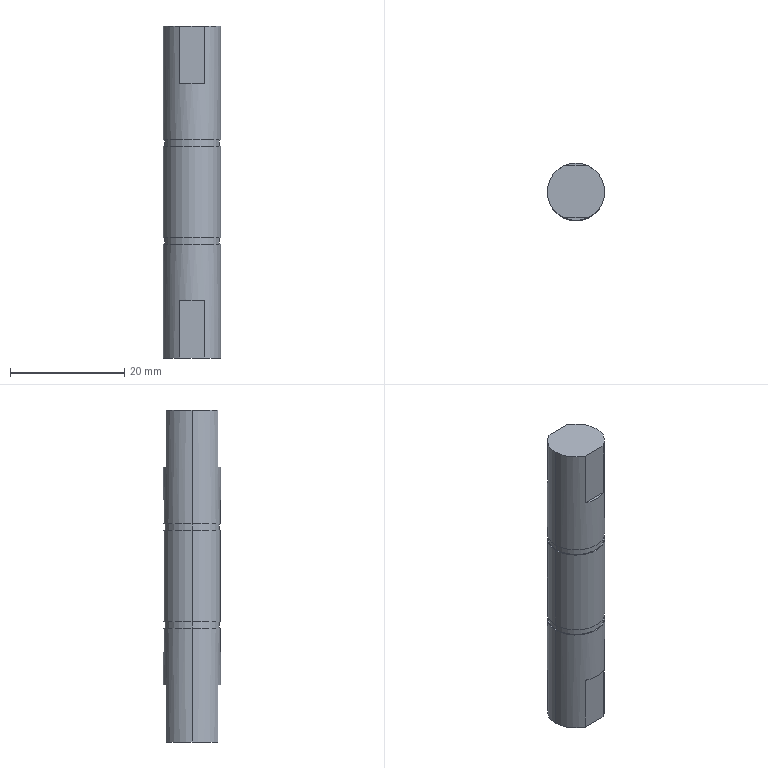Part | SolidWorks | features ICE 2, MirrorPattern 2, Extrusion 1, RefAxis 1 | 1 solid | 24 faces | box 10 x 10 x 58 mm | volume 4483 mm3 | plane 14 | cylinder 10 | commonest cylinder face diameters 10 x6 9.6 x4
STEP:
#1=CARTESIAN_POINT('',(4.8,0.,-9.1));
#2=VERTEX_POINT('',#1);
#3=CARTESIAN_POINT('',(-4.8,0.,-9.1));
#4=VERTEX_POINT('',#3);
#5=CARTESIAN_POINT('',(0.,0.,-9.1));
#6=DIRECTION('',(0.,0.,1.));
#7=DIRECTION('',(1.,0.,0.));
#8=AXIS2_PLACEMENT_3D('',#5,#6,#7);
#9=CIRCLE('',#8,4.8);
#10=EDGE_CURVE('',#2,#4,#9,.T.);
#11=ORIENTED_EDGE('',*,*,#10,.T.);
#12=CARTESIAN_POINT('',(-4.8,0.,-8.));
#13=VERTEX_POINT('',#12);
#14=CARTESIAN_POINT('',(-4.8,0.,-9.1));
#15=DIRECTION('',(0.,0.,1.));
#16=VECTOR('',#15,1000.);
#17=LINE('',#14,#16);
#18=EDGE_CURVE('',#4,#13,#17,.T.);
#19=ORIENTED_EDGE('',*,*,#18,.T.);
#20=CARTESIAN_POINT('',(4.8,0.,-8.));
#21=VERTEX_POINT('',#20);
#22=CARTESIAN_POINT('',(0.,0.,-8.));
#23=DIRECTION('',(0.,0.,1.));
#24=DIRECTION('',(1.,0.,0.));
#25=AXIS2_PLACEMENT_3D('',#22,#23,#24);
#26=CIRCLE('',#25,4.8);
#27=EDGE_CURVE('',#21,#13,#26,.T.);
#28=ORIENTED_EDGE('',*,*,#27,.F.);
#29=CARTESIAN_POINT('',(4.8,0.,-9.1));
#30=DIRECTION('',(0.,0.,1.));
#31=VECTOR('',#30,1000.);
#32=LINE('',#29,#31);
#33=EDGE_CURVE('',#2,#21,#32,.T.);
#34=ORIENTED_EDGE('',*,*,#33,.F.);
#35=EDGE_LOOP('',(#11,#19,#28,#34));
#36=FACE_OUTER_BOUND('',#35,.T.);
#37=CARTESIAN_POINT('',(0.,0.,-9.1));
#38=DIRECTION('',(0.,0.,1.));
#39=DIRECTION('',(1.,0.,0.));
#40=AXIS2_PLACEMENT_3D('',#37,#38,#39);
#41=CYLINDRICAL_SURFACE('',#40,4.8);
#42=ADVANCED_FACE('',(#36),#41,.T.);
#43=CARTESIAN_POINT('',(4.8,0.,9.1));
#44=VERTEX_POINT('',#43);
#45=CARTESIAN_POINT('',(-4.8,0.,9.1));
#46=VERTEX_POINT('',#45);
#47=CARTESIAN_POINT('',(0.,0.,9.1));
#48=DIRECTION('',(0.,0.,1.));
#49=DIRECTION('',(1.,0.,0.));
#50=AXIS2_PLACEMENT_3D('',#47,#48,#49);
#51=CIRCLE('',#50,4.8);
#52=EDGE_CURVE('',#44,#46,#51,.T.);
#53=ORIENTED_EDGE('',*,*,#52,.F.);
#54=CARTESIAN_POINT('',(4.8,0.,8.));
#55=VERTEX_POINT('',#54);
#56=CARTESIAN_POINT('',(4.8,0.,9.1));
#57=DIRECTION('',(0.,0.,-1.));
#58=VECTOR('',#57,1000.);
#59=LINE('',#56,#58);
#60=EDGE_CURVE('',#44,#55,#59,.T.);
#61=ORIENTED_EDGE('',*,*,#60,.T.);
#62=CARTESIAN_POINT('',(-4.8,0.,8.));
#63=VERTEX_POINT('',#62);
#64=CARTESIAN_POINT('',(0.,0.,8.));
#65=DIRECTION('',(0.,0.,1.));
#66=DIRECTION('',(1.,0.,0.));
#67=AXIS2_PLACEMENT_3D('',#64,#65,#66);
#68=CIRCLE('',#67,4.8);
#69=EDGE_CURVE('',#55,#63,#68,.T.);
#70=ORIENTED_EDGE('',*,*,#69,.T.);
#71=CARTESIAN_POINT('',(-4.8,0.,9.1));
#72=DIRECTION('',(0.,0.,-1.));
#73=VECTOR('',#72,1000.);
#74=LINE('',#71,#73);
#75=EDGE_CURVE('',#46,#63,#74,.T.);
#76=ORIENTED_EDGE('',*,*,#75,.F.);
#77=EDGE_LOOP('',(#53,#61,#70,#76));
#78=FACE_OUTER_BOUND('',#77,.T.);
#79=CARTESIAN_POINT('',(0.,0.,9.1));
#80=DIRECTION('',(0.,0.,-1.));
#81=DIRECTION('',(-1.,0.,0.));
#82=AXIS2_PLACEMENT_3D('',#79,#80,#81);
#83=CYLINDRICAL_SURFACE('',#82,4.8);
#84=ADVANCED_FACE('',(#78),#83,.T.);
#85=CARTESIAN_POINT('',(5.,0.,29.));
#86=VERTEX_POINT('',#85);
#87=CARTESIAN_POINT('',(2.179,4.5,29.));
#88=VERTEX_POINT('',#87);
#89=CARTESIAN_POINT('',(0.,0.,29.));
#90=DIRECTION('',(0.,0.,1.));
#91=DIRECTION('',(1.,0.,0.));
#92=AXIS2_PLACEMENT_3D('',#89,#90,#91);
#93=CIRCLE('',#92,5.);
#94=EDGE_CURVE('',#86,#88,#93,.T.);
#95=ORIENTED_EDGE('',*,*,#94,.F.);
#96=CARTESIAN_POINT('',(5.,0.,9.1));
#97=VERTEX_POINT('',#96);
#98=CARTESIAN_POINT('',(5.,0.,29.));
#99=DIRECTION('',(0.,0.,-1.));
#100=VECTOR('',#99,1000.);
#101=LINE('',#98,#100);
#102=EDGE_CURVE('',#86,#97,#101,.T.);
#103=ORIENTED_EDGE('',*,*,#102,.T.);
#104=CARTESIAN_POINT('',(-5.,0.,9.1));
#105=VERTEX_POINT('',#104);
#106=CARTESIAN_POINT('',(0.,0.,9.1));
#107=DIRECTION('',(0.,0.,1.));
#108=DIRECTION('',(1.,0.,0.));
#109=AXIS2_PLACEMENT_3D('',#106,#107,#108);
#110=CIRCLE('',#109,5.);
#111=EDGE_CURVE('',#97,#105,#110,.T.);
#112=ORIENTED_EDGE('',*,*,#111,.T.);
#113=CARTESIAN_POINT('',(-5.,0.,29.));
#114=VERTEX_POINT('',#113);
#115=CARTESIAN_POINT('',(-5.,0.,29.));
#116=DIRECTION('',(0.,0.,-1.));
#117=VECTOR('',#116,1000.);
#118=LINE('',#115,#117);
#119=EDGE_CURVE('',#114,#105,#118,.T.);
#120=ORIENTED_EDGE('',*,*,#119,.F.);
#121=CARTESIAN_POINT('',(-2.179,4.5,29.));
#122=VERTEX_POINT('',#121);
#123=CARTESIAN_POINT('',(0.,0.,29.));
#124=DIRECTION('',(0.,0.,1.));
#125=DIRECTION('',(1.,0.,0.));
#126=AXIS2_PLACEMENT_3D('',#123,#124,#125);
#127=CIRCLE('',#126,5.);
#128=EDGE_CURVE('',#122,#114,#127,.T.);
#129=ORIENTED_EDGE('',*,*,#128,.F.);
#130=CARTESIAN_POINT('',(-2.179,4.5,19.));
#131=VERTEX_POINT('',#130);
#132=CARTESIAN_POINT('',(-2.179,4.5,19.));
#133=DIRECTION('',(0.,0.,1.));
#134=VECTOR('',#133,1000.);
#135=LINE('',#132,#134);
#136=EDGE_CURVE('',#131,#122,#135,.T.);
#137=ORIENTED_EDGE('',*,*,#136,.F.);
#138=CARTESIAN_POINT('',(2.179,4.5,19.));
#139=VERTEX_POINT('',#138);
#140=CARTESIAN_POINT('',(0.,0.,19.));
#141=DIRECTION('',(0.,0.,1.));
#142=DIRECTION('',(1.,0.,0.));
#143=AXIS2_PLACEMENT_3D('',#140,#141,#142);
#144=CIRCLE('',#143,5.);
#145=EDGE_CURVE('',#139,#131,#144,.T.);
#146=ORIENTED_EDGE('',*,*,#145,.F.);
#147=CARTESIAN_POINT('',(2.179,4.5,19.));
#148=DIRECTION('',(0.,0.,1.));
#149=VECTOR('',#148,1000.);
#150=LINE('',#147,#149);
#151=EDGE_CURVE('',#139,#88,#150,.T.);
#152=ORIENTED_EDGE('',*,*,#151,.T.);
#153=EDGE_LOOP('',(#95,#103,#112,#120,#129,#137,#146,#152));
#154=FACE_OUTER_BOUND('',#153,.T.);
#155=CARTESIAN_POINT('',(0.,0.,29.));
#156=DIRECTION('',(0.,0.,-1.));
#157=DIRECTION('',(-1.,0.,0.));
#158=AXIS2_PLACEMENT_3D('',#155,#156,#157);
#159=CYLINDRICAL_SURFACE('',#158,5.);
#160=ADVANCED_FACE('',(#154),#159,.T.);
#161=CARTESIAN_POINT('',(5.,0.,8.));
#162=VERTEX_POINT('',#161);
#163=CARTESIAN_POINT('',(-5.,0.,8.));
#164=VERTEX_POINT('',#163);
#165=CARTESIAN_POINT('',(0.,0.,8.));
#166=DIRECTION('',(0.,0.,1.));
#167=DIRECTION('',(1.,0.,0.));
#168=AXIS2_PLACEMENT_3D('',#165,#166,#167);
#169=CIRCLE('',#168,5.);
#170=EDGE_CURVE('',#162,#164,#169,.T.);
#171=ORIENTED_EDGE('',*,*,#170,.F.);
#172=CARTESIAN_POINT('',(5.,0.,-8.));
#173=VERTEX_POINT('',#172);
#174=CARTESIAN_POINT('',(5.,0.,29.));
#175=DIRECTION('',(0.,0.,-1.));
#176=VECTOR('',#175,1000.);
#177=LINE('',#174,#176);
#178=EDGE_CURVE('',#162,#173,#177,.T.);
#179=ORIENTED_EDGE('',*,*,#178,.T.);
#180=CARTESIAN_POINT('',(-5.,0.,-8.));
#181=VERTEX_POINT('',#180);
#182=CARTESIAN_POINT('',(0.,0.,-8.));
#183=DIRECTION('',(0.,0.,1.));
#184=DIRECTION('',(1.,0.,0.));
#185=AXIS2_PLACEMENT_3D('',#182,#183,#184);
#186=CIRCLE('',#185,5.);
#187=EDGE_CURVE('',#173,#181,#186,.T.);
#188=ORIENTED_EDGE('',*,*,#187,.T.);
#189=CARTESIAN_POINT('',(-5.,0.,29.));
#190=DIRECTION('',(0.,0.,-1.));
#191=VECTOR('',#190,1000.);
#192=LINE('',#189,#191);
#193=EDGE_CURVE('',#164,#181,#192,.T.);
#194=ORIENTED_EDGE('',*,*,#193,.F.);
#195=EDGE_LOOP('',(#171,#179,#188,#194));
#196=FACE_OUTER_BOUND('',#195,.T.);
#197=CARTESIAN_POINT('',(0.,0.,29.));
#198=DIRECTION('',(0.,0.,-1.));
#199=DIRECTION('',(-1.,0.,0.));
#200=AXIS2_PLACEMENT_3D('',#197,#198,#199);
#201=CYLINDRICAL_SURFACE('',#200,5.);
#202=ADVANCED_FACE('',(#196),#201,.T.);
#203=CARTESIAN_POINT('',(5.,0.,-9.1));
#204=VERTEX_POINT('',#203);
#205=CARTESIAN_POINT('',(-5.,0.,-9.1));
#206=VERTEX_POINT('',#205);
#207=CARTESIAN_POINT('',(0.,0.,-9.1));
#208=DIRECTION('',(0.,0.,1.));
#209=DIRECTION('',(1.,0.,0.));
#210=AXIS2_PLACEMENT_3D('',#207,#208,#209);
#211=CIRCLE('',#210,5.);
#212=EDGE_CURVE('',#204,#206,#211,.T.);
#213=ORIENTED_EDGE('',*,*,#212,.F.);
#214=CARTESIAN_POINT('',(5.,0.,-29.));
#215=VERTEX_POINT('',#214);
#216=CARTESIAN_POINT('',(5.,0.,29.));
#217=DIRECTION('',(0.,0.,-1.));
#218=VECTOR('',#217,1000.);
#219=LINE('',#216,#218);
#220=EDGE_CURVE('',#204,#215,#219,.T.);
#221=ORIENTED_EDGE('',*,*,#220,.T.);
#222=CARTESIAN_POINT('',(2.179,4.5,-29.));
#223=VERTEX_POINT('',#222);
#224=CARTESIAN_POINT('',(0.,0.,-29.));
#225=DIRECTION('',(0.,0.,1.));
#226=DIRECTION('',(1.,0.,0.));
#227=AXIS2_PLACEMENT_3D('',#224,#225,#226);
#228=CIRCLE('',#227,5.);
#229=EDGE_CURVE('',#215,#223,#228,.T.);
#230=ORIENTED_EDGE('',*,*,#229,.T.);
#231=CARTESIAN_POINT('',(2.179,4.5,-19.));
#232=VERTEX_POINT('',#231);
#233=CARTESIAN_POINT('',(2.179,4.5,-19.));
#234=DIRECTION('',(0.,0.,-1.));
#235=VECTOR('',#234,1000.);
#236=LINE('',#233,#235);
#237=EDGE_CURVE('',#232,#223,#236,.T.);
#238=ORIENTED_EDGE('',*,*,#237,.F.);
#239=CARTESIAN_POINT('',(-2.179,4.5,-19.));
#240=VERTEX_POINT('',#239);
#241=CARTESIAN_POINT('',(0.,0.,-19.));
#242=DIRECTION('',(0.,0.,1.));
#243=DIRECTION('',(1.,0.,0.));
#244=AXIS2_PLACEMENT_3D('',#241,#242,#243);
#245=CIRCLE('',#244,5.);
#246=EDGE_CURVE('',#232,#240,#245,.T.);
#247=ORIENTED_EDGE('',*,*,#246,.T.);
#248=CARTESIAN_POINT('',(-2.179,4.5,-29.));
#249=VERTEX_POINT('',#248);
#250=CARTESIAN_POINT('',(-2.179,4.5,-19.));
#251=DIRECTION('',(0.,0.,-1.));
#252=VECTOR('',#251,1000.);
#253=LINE('',#250,#252);
#254=EDGE_CURVE('',#240,#249,#253,.T.);
#255=ORIENTED_EDGE('',*,*,#254,.T.);
#256=CARTESIAN_POINT('',(-5.,0.,-29.));
#257=VERTEX_POINT('',#256);
#258=CARTESIAN_POINT('',(0.,0.,-29.));
#259=DIRECTION('',(0.,0.,1.));
#260=DIRECTION('',(1.,0.,0.));
#261=AXIS2_PLACEMENT_3D('',#258,#259,#260);
#262=CIRCLE('',#261,5.);
#263=EDGE_CURVE('',#249,#257,#262,.T.);
#264=ORIENTED_EDGE('',*,*,#263,.T.);
#265=CARTESIAN_POINT('',(-5.,0.,29.));
#266=DIRECTION('',(0.,0.,-1.));
#267=VECTOR('',#266,1000.);
#268=LINE('',#265,#267);
#269=EDGE_CURVE('',#206,#257,#268,.T.);
#270=ORIENTED_EDGE('',*,*,#269,.F.);
#271=EDGE_LOOP('',(#213,#221,#230,#238,#247,#255,#264,#270));
#272=FACE_OUTER_BOUND('',#271,.T.);
#273=CARTESIAN_POINT('',(0.,0.,29.));
#274=DIRECTION('',(0.,0.,-1.));
#275=DIRECTION('',(-1.,0.,0.));
#276=AXIS2_PLACEMENT_3D('',#273,#274,#275);
#277=CYLINDRICAL_SURFACE('',#276,5.);
#278=ADVANCED_FACE('',(#272),#277,.T.);
#279=CARTESIAN_POINT('',(-2.179,4.5,-29.));
#280=DIRECTION('',(1.,0.,0.));
#281=VECTOR('',#280,1000.);
#282=LINE('',#279,#281);
#283=EDGE_CURVE('',#249,#223,#282,.T.);
#284=ORIENTED_EDGE('',*,*,#283,.T.);
#285=ORIENTED_EDGE('',*,*,#229,.F.);
#286=CARTESIAN_POINT('',(2.179,-4.5,-29.));
#287=VERTEX_POINT('',#286);
#288=CARTESIAN_POINT('',(0.,0.,-29.));
#289=DIRECTION('',(0.,0.,1.));
#290=DIRECTION('',(1.,0.,0.));
#291=AXIS2_PLACEMENT_3D('',#288,#289,#290);
#292=CIRCLE('',#291,5.);
#293=EDGE_CURVE('',#287,#215,#292,.T.);
#294=ORIENTED_EDGE('',*,*,#293,.F.);
#295=CARTESIAN_POINT('',(-2.179,-4.5,-29.));
#296=VERTEX_POINT('',#295);
#297=CARTESIAN_POINT('',(-2.179,-4.5,-29.));
#298=DIRECTION('',(-1.,0.,0.));
#299=VECTOR('',#298,1000.);
#300=LINE('',#297,#299);
#301=EDGE_CURVE('',#287,#296,#300,.T.);
#302=ORIENTED_EDGE('',*,*,#301,.T.);
#303=CARTESIAN_POINT('',(0.,0.,-29.));
#304=DIRECTION('',(0.,0.,1.));
#305=DIRECTION('',(1.,0.,0.));
#306=AXIS2_PLACEMENT_3D('',#303,#304,#305);
#307=CIRCLE('',#306,5.);
#308=EDGE_CURVE('',#257,#296,#307,.T.);
#309=ORIENTED_EDGE('',*,*,#308,.F.);
#310=ORIENTED_EDGE('',*,*,#263,.F.);
#311=EDGE_LOOP('',(#284,#285,#294,#302,#309,#310));
#312=FACE_OUTER_BOUND('',#311,.T.);
#313=CARTESIAN_POINT('',(0.,0.,-29.));
#314=DIRECTION('',(0.,0.,1.));
#315=DIRECTION('',(1.,0.,0.));
#316=AXIS2_PLACEMENT_3D('',#313,#314,#315);
#317=PLANE('',#316);
#318=ADVANCED_FACE('',(#312),#317,.F.);
#319=ORIENTED_EDGE('',*,*,#220,.F.);
#320=CARTESIAN_POINT('',(0.,0.,-9.1));
#321=DIRECTION('',(0.,0.,1.));
#322=DIRECTION('',(1.,0.,0.));
#323=AXIS2_PLACEMENT_3D('',#320,#321,#322);
#324=CIRCLE('',#323,5.);
#325=EDGE_CURVE('',#206,#204,#324,.T.);
#326=ORIENTED_EDGE('',*,*,#325,.F.);
#327=ORIENTED_EDGE('',*,*,#269,.T.);
#328=ORIENTED_EDGE('',*,*,#308,.T.);
#329=CARTESIAN_POINT('',(-2.179,-4.5,-19.));
#330=VERTEX_POINT('',#329);
#331=CARTESIAN_POINT('',(-2.179,-4.5,-19.));
#332=DIRECTION('',(0.,0.,-1.));
#333=VECTOR('',#332,1000.);
#334=LINE('',#331,#333);
#335=EDGE_CURVE('',#330,#296,#334,.T.);
#336=ORIENTED_EDGE('',*,*,#335,.F.);
#337=CARTESIAN_POINT('',(2.179,-4.5,-19.));
#338=VERTEX_POINT('',#337);
#339=CARTESIAN_POINT('',(0.,0.,-19.));
#340=DIRECTION('',(0.,0.,1.));
#341=DIRECTION('',(1.,0.,0.));
#342=AXIS2_PLACEMENT_3D('',#339,#340,#341);
#343=CIRCLE('',#342,5.);
#344=EDGE_CURVE('',#330,#338,#343,.T.);
#345=ORIENTED_EDGE('',*,*,#344,.T.);
#346=CARTESIAN_POINT('',(2.179,-4.5,-19.));
#347=DIRECTION('',(0.,0.,-1.));
#348=VECTOR('',#347,1000.);
#349=LINE('',#346,#348);
#350=EDGE_CURVE('',#338,#287,#349,.T.);
#351=ORIENTED_EDGE('',*,*,#350,.T.);
#352=ORIENTED_EDGE('',*,*,#293,.T.);
#353=EDGE_LOOP('',(#319,#326,#327,#328,#336,#345,#351,#352));
#354=FACE_OUTER_BOUND('',#353,.T.);
#355=CARTESIAN_POINT('',(0.,0.,29.));
#356=DIRECTION('',(0.,0.,-1.));
#357=DIRECTION('',(-1.,0.,0.));
#358=AXIS2_PLACEMENT_3D('',#355,#356,#357);
#359=CYLINDRICAL_SURFACE('',#358,5.);
#360=ADVANCED_FACE('',(#354),#359,.T.);
#361=ORIENTED_EDGE('',*,*,#178,.F.);
#362=CARTESIAN_POINT('',(0.,0.,8.));
#363=DIRECTION('',(0.,0.,1.));
#364=DIRECTION('',(1.,0.,0.));
#365=AXIS2_PLACEMENT_3D('',#362,#363,#364);
#366=CIRCLE('',#365,5.);
#367=EDGE_CURVE('',#164,#162,#366,.T.);
#368=ORIENTED_EDGE('',*,*,#367,.F.);
#369=ORIENTED_EDGE('',*,*,#193,.T.);
#370=CARTESIAN_POINT('',(0.,0.,-8.));
#371=DIRECTION('',(0.,0.,1.));
#372=DIRECTION('',(1.,0.,0.));
#373=AXIS2_PLACEMENT_3D('',#370,#371,#372);
#374=CIRCLE('',#373,5.);
#375=EDGE_CURVE('',#181,#173,#374,.T.);
#376=ORIENTED_EDGE('',*,*,#375,.T.);
#377=EDGE_LOOP('',(#361,#368,#369,#376));
#378=FACE_OUTER_BOUND('',#377,.T.);
#379=CARTESIAN_POINT('',(0.,0.,29.));
#380=DIRECTION('',(0.,0.,-1.));
#381=DIRECTION('',(-1.,0.,0.));
#382=AXIS2_PLACEMENT_3D('',#379,#380,#381);
#383=CYLINDRICAL_SURFACE('',#382,5.);
#384=ADVANCED_FACE('',(#378),#383,.T.);
#385=ORIENTED_EDGE('',*,*,#102,.F.);
#386=CARTESIAN_POINT('',(2.179,-4.5,29.));
#387=VERTEX_POINT('',#386);
#388=CARTESIAN_POINT('',(0.,0.,29.));
#389=DIRECTION('',(0.,0.,1.));
#390=DIRECTION('',(1.,0.,0.));
#391=AXIS2_PLACEMENT_3D('',#388,#389,#390);
#392=CIRCLE('',#391,5.);
#393=EDGE_CURVE('',#387,#86,#392,.T.);
#394=ORIENTED_EDGE('',*,*,#393,.F.);
#395=CARTESIAN_POINT('',(2.179,-4.5,19.));
#396=VERTEX_POINT('',#395);
#397=CARTESIAN_POINT('',(2.179,-4.5,19.));
#398=DIRECTION('',(0.,0.,1.));
#399=VECTOR('',#398,1000.);
#400=LINE('',#397,#399);
#401=EDGE_CURVE('',#396,#387,#400,.T.);
#402=ORIENTED_EDGE('',*,*,#401,.F.);
#403=CARTESIAN_POINT('',(-2.179,-4.5,19.));
#404=VERTEX_POINT('',#403);
#405=CARTESIAN_POINT('',(0.,0.,19.));
#406=DIRECTION('',(0.,0.,1.));
#407=DIRECTION('',(1.,0.,0.));
#408=AXIS2_PLACEMENT_3D('',#405,#406,#407);
#409=CIRCLE('',#408,5.);
#410=EDGE_CURVE('',#404,#396,#409,.T.);
#411=ORIENTED_EDGE('',*,*,#410,.F.);
#412=CARTESIAN_POINT('',(-2.179,-4.5,29.));
#413=VERTEX_POINT('',#412);
#414=CARTESIAN_POINT('',(-2.179,-4.5,19.));
#415=DIRECTION('',(0.,0.,1.));
#416=VECTOR('',#415,1000.);
#417=LINE('',#414,#416);
#418=EDGE_CURVE('',#404,#413,#417,.T.);
#419=ORIENTED_EDGE('',*,*,#418,.T.);
#420=CARTESIAN_POINT('',(0.,0.,29.));
#421=DIRECTION('',(0.,0.,1.));
#422=DIRECTION('',(1.,0.,0.));
#423=AXIS2_PLACEMENT_3D('',#420,#421,#422);
#424=CIRCLE('',#423,5.);
#425=EDGE_CURVE('',#114,#413,#424,.T.);
#426=ORIENTED_EDGE('',*,*,#425,.F.);
#427=ORIENTED_EDGE('',*,*,#119,.T.);
#428=CARTESIAN_POINT('',(0.,0.,9.1));
#429=DIRECTION('',(0.,0.,1.));
#430=DIRECTION('',(1.,0.,0.));
#431=AXIS2_PLACEMENT_3D('',#428,#429,#430);
#432=CIRCLE('',#431,5.);
#433=EDGE_CURVE('',#105,#97,#432,.T.);
#434=ORIENTED_EDGE('',*,*,#433,.T.);
#435=EDGE_LOOP('',(#385,#394,#402,#411,#419,#426,#427,#434));
#436=FACE_OUTER_BOUND('',#435,.T.);
#437=CARTESIAN_POINT('',(0.,0.,29.));
#438=DIRECTION('',(0.,0.,-1.));
#439=DIRECTION('',(-1.,0.,0.));
#440=AXIS2_PLACEMENT_3D('',#437,#438,#439);
#441=CYLINDRICAL_SURFACE('',#440,5.);
#442=ADVANCED_FACE('',(#436),#441,.T.);
#443=CARTESIAN_POINT('',(-2.179,4.5,29.));
#444=DIRECTION('',(1.,0.,0.));
#445=VECTOR('',#444,1000.);
#446=LINE('',#443,#445);
#447=EDGE_CURVE('',#122,#88,#446,.T.);
#448=ORIENTED_EDGE('',*,*,#447,.F.);
#449=ORIENTED_EDGE('',*,*,#128,.T.);
#450=ORIENTED_EDGE('',*,*,#425,.T.);
#451=CARTESIAN_POINT('',(-2.179,-4.5,29.));
#452=DIRECTION('',(-1.,0.,0.));
#453=VECTOR('',#452,1000.);
#454=LINE('',#451,#453);
#455=EDGE_CURVE('',#387,#413,#454,.T.);
#456=ORIENTED_EDGE('',*,*,#455,.F.);
#457=ORIENTED_EDGE('',*,*,#393,.T.);
#458=ORIENTED_EDGE('',*,*,#94,.T.);
#459=EDGE_LOOP('',(#448,#449,#450,#456,#457,#458));
#460=FACE_OUTER_BOUND('',#459,.T.);
#461=CARTESIAN_POINT('',(0.,0.,29.));
#462=DIRECTION('',(0.,0.,1.));
#463=DIRECTION('',(1.,0.,0.));
#464=AXIS2_PLACEMENT_3D('',#461,#462,#463);
#465=PLANE('',#464);
#466=ADVANCED_FACE('',(#460),#465,.T.);
#467=ORIENTED_EDGE('',*,*,#433,.F.);
#468=ORIENTED_EDGE('',*,*,#111,.F.);
#469=EDGE_LOOP('',(#467,#468));
#470=FACE_OUTER_BOUND('',#469,.T.);
#471=CARTESIAN_POINT('',(0.,0.,9.1));
#472=DIRECTION('',(0.,0.,1.));
#473=DIRECTION('',(1.,0.,0.));
#474=AXIS2_PLACEMENT_3D('',#471,#472,#473);
#475=CIRCLE('',#474,4.8);
#476=EDGE_CURVE('',#46,#44,#475,.T.);
#477=ORIENTED_EDGE('',*,*,#476,.T.);
#478=ORIENTED_EDGE('',*,*,#52,.T.);
#479=EDGE_LOOP('',(#477,#478));
#480=FACE_BOUND('',#479,.T.);
#481=CARTESIAN_POINT('',(0.,0.,9.1));
#482=DIRECTION('',(0.,0.,1.));
#483=DIRECTION('',(1.,0.,0.));
#484=AXIS2_PLACEMENT_3D('',#481,#482,#483);
#485=PLANE('',#484);
#486=ADVANCED_FACE('',(#470,#480),#485,.F.);
#487=ORIENTED_EDGE('',*,*,#367,.T.);
#488=ORIENTED_EDGE('',*,*,#170,.T.);
#489=EDGE_LOOP('',(#487,#488));
#490=FACE_OUTER_BOUND('',#489,.T.);
#491=CARTESIAN_POINT('',(0.,0.,8.));
#492=DIRECTION('',(0.,0.,1.));
#493=DIRECTION('',(1.,0.,0.));
#494=AXIS2_PLACEMENT_3D('',#491,#492,#493);
#495=CIRCLE('',#494,4.8);
#496=EDGE_CURVE('',#63,#55,#495,.T.);
#497=ORIENTED_EDGE('',*,*,#496,.F.);
#498=ORIENTED_EDGE('',*,*,#69,.F.);
#499=EDGE_LOOP('',(#497,#498));
#500=FACE_BOUND('',#499,.T.);
#501=CARTESIAN_POINT('',(0.,0.,8.));
#502=DIRECTION('',(0.,0.,1.));
#503=DIRECTION('',(1.,0.,0.));
#504=AXIS2_PLACEMENT_3D('',#501,#502,#503);
#505=PLANE('',#504);
#506=ADVANCED_FACE('',(#490,#500),#505,.T.);
#507=ORIENTED_EDGE('',*,*,#60,.F.);
#508=ORIENTED_EDGE('',*,*,#476,.F.);
#509=ORIENTED_EDGE('',*,*,#75,.T.);
#510=ORIENTED_EDGE('',*,*,#496,.T.);
#511=EDGE_LOOP('',(#507,#508,#509,#510));
#512=FACE_OUTER_BOUND('',#511,.T.);
#513=CARTESIAN_POINT('',(0.,0.,9.1));
#514=DIRECTION('',(0.,0.,-1.));
#515=DIRECTION('',(-1.,0.,0.));
#516=AXIS2_PLACEMENT_3D('',#513,#514,#515);
#517=CYLINDRICAL_SURFACE('',#516,4.8);
#518=ADVANCED_FACE('',(#512),#517,.T.);
#519=ORIENTED_EDGE('',*,*,#10,.F.);
#520=CARTESIAN_POINT('',(0.,0.,-9.1));
#521=DIRECTION('',(0.,0.,1.));
#522=DIRECTION('',(1.,0.,0.));
#523=AXIS2_PLACEMENT_3D('',#520,#521,#522);
#524=CIRCLE('',#523,4.8);
#525=EDGE_CURVE('',#4,#2,#524,.T.);
#526=ORIENTED_EDGE('',*,*,#525,.F.);
#527=EDGE_LOOP('',(#519,#526));
#528=FACE_BOUND('',#527,.T.);
#529=ORIENTED_EDGE('',*,*,#325,.T.);
#530=ORIENTED_EDGE('',*,*,#212,.T.);
#531=EDGE_LOOP('',(#529,#530));
#532=FACE_OUTER_BOUND('',#531,.T.);
#533=CARTESIAN_POINT('',(0.,0.,-9.1));
#534=DIRECTION('',(0.,0.,-1.));
#535=DIRECTION('',(1.,0.,0.));
#536=AXIS2_PLACEMENT_3D('',#533,#534,#535);
#537=PLANE('',#536);
#538=ADVANCED_FACE('',(#528,#532),#537,.F.);
#539=ORIENTED_EDGE('',*,*,#27,.T.);
#540=CARTESIAN_POINT('',(0.,0.,-8.));
#541=DIRECTION('',(0.,0.,1.));
#542=DIRECTION('',(1.,0.,0.));
#543=AXIS2_PLACEMENT_3D('',#540,#541,#542);
#544=CIRCLE('',#543,4.8);
#545=EDGE_CURVE('',#13,#21,#544,.T.);
#546=ORIENTED_EDGE('',*,*,#545,.T.);
#547=EDGE_LOOP('',(#539,#546));
#548=FACE_BOUND('',#547,.T.);
#549=ORIENTED_EDGE('',*,*,#375,.F.);
#550=ORIENTED_EDGE('',*,*,#187,.F.);
#551=EDGE_LOOP('',(#549,#550));
#552=FACE_OUTER_BOUND('',#551,.T.);
#553=CARTESIAN_POINT('',(0.,0.,-8.));
#554=DIRECTION('',(0.,0.,-1.));
#555=DIRECTION('',(1.,0.,0.));
#556=AXIS2_PLACEMENT_3D('',#553,#554,#555);
#557=PLANE('',#556);
#558=ADVANCED_FACE('',(#548,#552),#557,.T.);
#559=ORIENTED_EDGE('',*,*,#18,.F.);
#560=ORIENTED_EDGE('',*,*,#525,.T.);
#561=ORIENTED_EDGE('',*,*,#33,.T.);
#562=ORIENTED_EDGE('',*,*,#545,.F.);
#563=EDGE_LOOP('',(#559,#560,#561,#562));
#564=FACE_OUTER_BOUND('',#563,.T.);
#565=CARTESIAN_POINT('',(0.,0.,-9.1));
#566=DIRECTION('',(0.,0.,1.));
#567=DIRECTION('',(1.,0.,0.));
#568=AXIS2_PLACEMENT_3D('',#565,#566,#567);
#569=CYLINDRICAL_SURFACE('',#568,4.8);
#570=ADVANCED_FACE('',(#564),#569,.T.);
#571=ORIENTED_EDGE('',*,*,#455,.T.);
#572=ORIENTED_EDGE('',*,*,#418,.F.);
#573=CARTESIAN_POINT('',(-2.179,-4.5,19.));
#574=DIRECTION('',(-1.,0.,0.));
#575=VECTOR('',#574,1000.);
#576=LINE('',#573,#575);
#577=EDGE_CURVE('',#396,#404,#576,.T.);
#578=ORIENTED_EDGE('',*,*,#577,.F.);
#579=ORIENTED_EDGE('',*,*,#401,.T.);
#580=EDGE_LOOP('',(#571,#572,#578,#579));
#581=FACE_OUTER_BOUND('',#580,.T.);
#582=CARTESIAN_POINT('',(-2.179,-4.5,19.));
#583=DIRECTION('',(0.,1.,0.));
#584=DIRECTION('',(0.,0.,1.));
#585=AXIS2_PLACEMENT_3D('',#582,#583,#584);
#586=PLANE('',#585);
#587=ADVANCED_FACE('',(#581),#586,.F.);
#588=ORIENTED_EDGE('',*,*,#410,.T.);
#589=ORIENTED_EDGE('',*,*,#577,.T.);
#590=EDGE_LOOP('',(#588,#589));
#591=FACE_OUTER_BOUND('',#590,.T.);
#592=CARTESIAN_POINT('',(0.,0.,19.));
#593=DIRECTION('',(0.,0.,1.));
#594=DIRECTION('',(1.,0.,0.));
#595=AXIS2_PLACEMENT_3D('',#592,#593,#594);
#596=PLANE('',#595);
#597=ADVANCED_FACE('',(#591),#596,.T.);
#598=ORIENTED_EDGE('',*,*,#447,.T.);
#599=ORIENTED_EDGE('',*,*,#151,.F.);
#600=CARTESIAN_POINT('',(-2.179,4.5,19.));
#601=DIRECTION('',(1.,0.,0.));
#602=VECTOR('',#601,1000.);
#603=LINE('',#600,#602);
#604=EDGE_CURVE('',#131,#139,#603,.T.);
#605=ORIENTED_EDGE('',*,*,#604,.F.);
#606=ORIENTED_EDGE('',*,*,#136,.T.);
#607=EDGE_LOOP('',(#598,#599,#605,#606));
#608=FACE_OUTER_BOUND('',#607,.T.);
#609=CARTESIAN_POINT('',(-2.179,4.5,19.));
#610=DIRECTION('',(0.,-1.,0.));
#611=DIRECTION('',(0.,0.,-1.));
#612=AXIS2_PLACEMENT_3D('',#609,#610,#611);
#613=PLANE('',#612);
#614=ADVANCED_FACE('',(#608),#613,.F.);
#615=ORIENTED_EDGE('',*,*,#145,.T.);
#616=ORIENTED_EDGE('',*,*,#604,.T.);
#617=EDGE_LOOP('',(#615,#616));
#618=FACE_OUTER_BOUND('',#617,.T.);
#619=CARTESIAN_POINT('',(0.,0.,19.));
#620=DIRECTION('',(0.,0.,1.));
#621=DIRECTION('',(1.,0.,0.));
#622=AXIS2_PLACEMENT_3D('',#619,#620,#621);
#623=PLANE('',#622);
#624=ADVANCED_FACE('',(#618),#623,.T.);
#625=ORIENTED_EDGE('',*,*,#301,.F.);
#626=ORIENTED_EDGE('',*,*,#350,.F.);
#627=CARTESIAN_POINT('',(-2.179,-4.5,-19.));
#628=DIRECTION('',(-1.,0.,0.));
#629=VECTOR('',#628,1000.);
#630=LINE('',#627,#629);
#631=EDGE_CURVE('',#338,#330,#630,.T.);
#632=ORIENTED_EDGE('',*,*,#631,.T.);
#633=ORIENTED_EDGE('',*,*,#335,.T.);
#634=EDGE_LOOP('',(#625,#626,#632,#633));
#635=FACE_OUTER_BOUND('',#634,.T.);
#636=CARTESIAN_POINT('',(-2.179,-4.5,-19.));
#637=DIRECTION('',(0.,-1.,0.));
#638=DIRECTION('',(0.,0.,-1.));
#639=AXIS2_PLACEMENT_3D('',#636,#637,#638);
#640=PLANE('',#639);
#641=ADVANCED_FACE('',(#635),#640,.T.);
#642=ORIENTED_EDGE('',*,*,#344,.F.);
#643=ORIENTED_EDGE('',*,*,#631,.F.);
#644=EDGE_LOOP('',(#642,#643));
#645=FACE_OUTER_BOUND('',#644,.T.);
#646=CARTESIAN_POINT('',(0.,0.,-19.));
#647=DIRECTION('',(0.,0.,-1.));
#648=DIRECTION('',(1.,0.,0.));
#649=AXIS2_PLACEMENT_3D('',#646,#647,#648);
#650=PLANE('',#649);
#651=ADVANCED_FACE('',(#645),#650,.T.);
#652=ORIENTED_EDGE('',*,*,#283,.F.);
#653=ORIENTED_EDGE('',*,*,#254,.F.);
#654=CARTESIAN_POINT('',(-2.179,4.5,-19.));
#655=DIRECTION('',(1.,0.,0.));
#656=VECTOR('',#655,1000.);
#657=LINE('',#654,#656);
#658=EDGE_CURVE('',#240,#232,#657,.T.);
#659=ORIENTED_EDGE('',*,*,#658,.T.);
#660=ORIENTED_EDGE('',*,*,#237,.T.);
#661=EDGE_LOOP('',(#652,#653,#659,#660));
#662=FACE_OUTER_BOUND('',#661,.T.);
#663=CARTESIAN_POINT('',(-2.179,4.5,-19.));
#664=DIRECTION('',(0.,1.,0.));
#665=DIRECTION('',(0.,0.,1.));
#666=AXIS2_PLACEMENT_3D('',#663,#664,#665);
#667=PLANE('',#666);
#668=ADVANCED_FACE('',(#662),#667,.T.);
#669=ORIENTED_EDGE('',*,*,#246,.F.);
#670=ORIENTED_EDGE('',*,*,#658,.F.);
#671=EDGE_LOOP('',(#669,#670));
#672=FACE_OUTER_BOUND('',#671,.T.);
#673=CARTESIAN_POINT('',(0.,0.,-19.));
#674=DIRECTION('',(0.,0.,-1.));
#675=DIRECTION('',(1.,0.,0.));
#676=AXIS2_PLACEMENT_3D('',#673,#674,#675);
#677=PLANE('',#676);
#678=ADVANCED_FACE('',(#672),#677,.T.);
#679=CLOSED_SHELL('',(#42,#84,#160,#202,#278,#318,#360,#384,#442,#466,#486,#506,#518,#538,#558,#570,#587,#597,#614,#624,#641,#651,#668,#678));
#680=MANIFOLD_SOLID_BREP('',#679);
#681=CARTESIAN_POINT('',(0.,0.,0.));
#682=DIRECTION('',(0.,0.,1.));
#683=DIRECTION('',(1.,0.,0.));
#684=AXIS2_PLACEMENT_3D('',#681,#682,#683);
#685=(LENGTH_UNIT()NAMED_UNIT(*)SI_UNIT(.MILLI.,.METRE.));
#686=UNCERTAINTY_MEASURE_WITH_UNIT(LENGTH_MEASURE(0.00001),#685,'','');
#687=(NAMED_UNIT(*)PLANE_ANGLE_UNIT()SI_UNIT($,.RADIAN.));
#688=(NAMED_UNIT(*)SI_UNIT($,.STERADIAN.)SOLID_ANGLE_UNIT());
#689=(GEOMETRIC_REPRESENTATION_CONTEXT(3)GLOBAL_UNCERTAINTY_ASSIGNED_CONTEXT((#686))GLOBAL_UNIT_ASSIGNED_CONTEXT((#685,#687,#688))REPRESENTATION_CONTEXT('',''));
#690=ADVANCED_BREP_SHAPE_REPRESENTATION('',(#680,#684),#689);